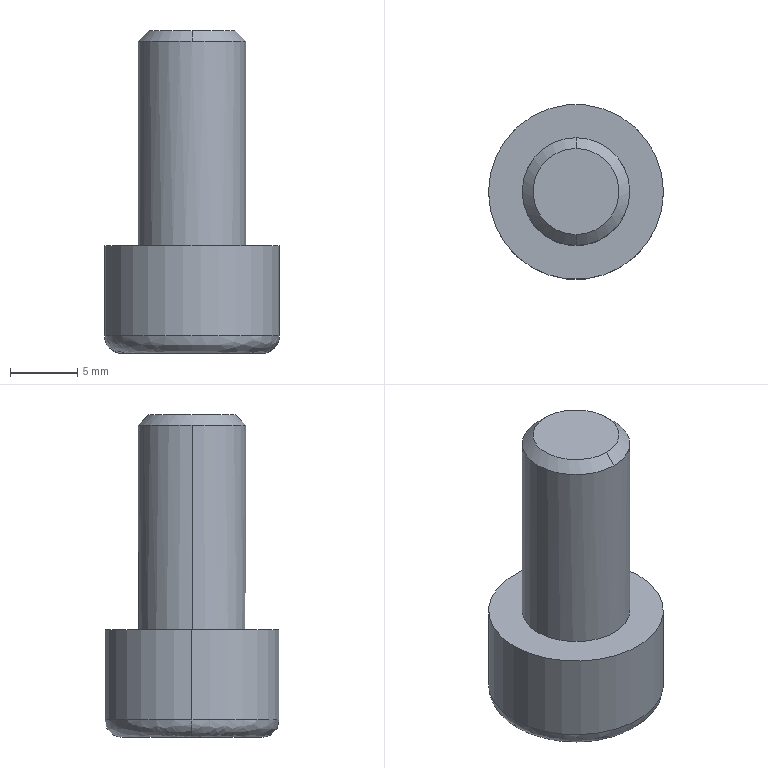Part | STEP file | HJLE-YZS-M8X16_LE0724153021 | 1 solid | 25 faces | box 13 x 13 x 24 mm | volume 1703 mm3 | plane 15 | cylinder 4 | cone 4 | spline 2 | commonest cylinder face diameters 8 x2 13 x2
STEP:
#1=CARTESIAN_POINT('',(-6.5,0.,-6.7));
#2=VERTEX_POINT('',#1);
#3=CARTESIAN_POINT('',(6.5,0.,-6.7));
#4=VERTEX_POINT('',#3);
#5=CARTESIAN_POINT('',(0.,0.,-6.7));
#6=DIRECTION('',(0.,0.,1.));
#7=DIRECTION('',(1.,0.,0.));
#8=AXIS2_PLACEMENT_3D('',#5,#6,#7);
#9=CIRCLE('',#8,6.5);
#10=EDGE_CURVE('',#2,#4,#9,.T.);
#11=ORIENTED_EDGE('',*,*,#10,.F.);
#12=CARTESIAN_POINT('',(-5.2,0.,-8.));
#13=VERTEX_POINT('',#12);
#14=CARTESIAN_POINT('',(-5.2,0.,-6.7));
#15=DIRECTION('',(0.,-1.,0.));
#16=DIRECTION('',(-1.,0.,0.));
#17=AXIS2_PLACEMENT_3D('',#14,#15,#16);
#18=CIRCLE('',#17,1.3);
#19=EDGE_CURVE('',#2,#13,#18,.T.);
#20=ORIENTED_EDGE('',*,*,#19,.T.);
#21=CARTESIAN_POINT('',(5.2,0.,-8.));
#22=VERTEX_POINT('',#21);
#23=CARTESIAN_POINT('',(-5.2,0.,-8.));
#24=CARTESIAN_POINT('',(-5.2,-10.4,-8.));
#25=CARTESIAN_POINT('',(5.2,-10.4,-8.));
#26=CARTESIAN_POINT('',(5.2,0.,-8.));
#27=(BOUNDED_CURVE()B_SPLINE_CURVE(3,(#23,#24,#25,#26),.UNSPECIFIED.,.F.,.F.)B_SPLINE_CURVE_WITH_KNOTS((4,4),(0.,1.),.UNSPECIFIED.)CURVE()GEOMETRIC_REPRESENTATION_ITEM()RATIONAL_B_SPLINE_CURVE((1.,0.3333,0.3333,1.))REPRESENTATION_ITEM(''));
#28=EDGE_CURVE('',#13,#22,#27,.T.);
#29=ORIENTED_EDGE('',*,*,#28,.T.);
#30=CARTESIAN_POINT('',(5.2,0.,-6.7));
#31=DIRECTION('',(0.,1.,0.));
#32=DIRECTION('',(1.,0.,0.));
#33=AXIS2_PLACEMENT_3D('',#30,#31,#32);
#34=CIRCLE('',#33,1.3);
#35=EDGE_CURVE('',#4,#22,#34,.T.);
#36=ORIENTED_EDGE('',*,*,#35,.F.);
#37=EDGE_LOOP('',(#11,#20,#29,#36));
#38=FACE_OUTER_BOUND('',#37,.T.);
#39=CARTESIAN_POINT('',(-6.5,0.,-6.7));
#40=CARTESIAN_POINT('',(-6.5,-13.,-6.7));
#41=CARTESIAN_POINT('',(6.5,-13.,-6.7));
#42=CARTESIAN_POINT('',(6.5,0.,-6.7));
#43=CARTESIAN_POINT('',(-6.5,0.,-7.462));
#44=CARTESIAN_POINT('',(-6.5,-13.,-7.462));
#45=CARTESIAN_POINT('',(6.5,-13.,-7.462));
#46=CARTESIAN_POINT('',(6.5,0.,-7.462));
#47=CARTESIAN_POINT('',(-5.962,0.,-8.));
#48=CARTESIAN_POINT('',(-5.962,-11.923,-8.));
#49=CARTESIAN_POINT('',(5.962,-11.923,-8.));
#50=CARTESIAN_POINT('',(5.962,0.,-8.));
#51=CARTESIAN_POINT('',(-5.2,0.,-8.));
#52=CARTESIAN_POINT('',(-5.2,-10.4,-8.));
#53=CARTESIAN_POINT('',(5.2,-10.4,-8.));
#54=CARTESIAN_POINT('',(5.2,0.,-8.));
#55=(BOUNDED_SURFACE()B_SPLINE_SURFACE(3,3,((#39,#40,#41,#42),(#43,#44,#45,#46),(#47,#48,#49,#50),(#51,#52,#53,#54)),.UNSPECIFIED.,.F.,.F.,.F.)B_SPLINE_SURFACE_WITH_KNOTS((4,4),(4,4),(0.,1.),(0.,1.),.UNSPECIFIED.)GEOMETRIC_REPRESENTATION_ITEM()RATIONAL_B_SPLINE_SURFACE(((1.,0.3333,0.3333,1.),(0.8047,0.2682,0.2682,0.8047),(0.8047,0.2682,0.2682,0.8047),(1.,0.3333,0.3333,1.)))REPRESENTATION_ITEM('')SURFACE());
#56=ADVANCED_FACE('',(#38),#55,.T.);
#57=CARTESIAN_POINT('',(0.,4.,15.2));
#58=VERTEX_POINT('',#57);
#59=CARTESIAN_POINT('',(4.,0.,15.2));
#60=VERTEX_POINT('',#59);
#61=CARTESIAN_POINT('',(0.,0.,15.2));
#62=DIRECTION('',(0.,0.,-1.));
#63=DIRECTION('',(-1.,0.,0.));
#64=AXIS2_PLACEMENT_3D('',#61,#62,#63);
#65=CIRCLE('',#64,4.);
#66=EDGE_CURVE('',#58,#60,#65,.T.);
#67=ORIENTED_EDGE('',*,*,#66,.T.);
#68=CARTESIAN_POINT('',(4.,0.,0.));
#69=VERTEX_POINT('',#68);
#70=CARTESIAN_POINT('',(4.,0.,16.));
#71=DIRECTION('',(0.,0.,-1.));
#72=VECTOR('',#71,1000.);
#73=LINE('',#70,#72);
#74=EDGE_CURVE('',#60,#69,#73,.T.);
#75=ORIENTED_EDGE('',*,*,#74,.T.);
#76=CARTESIAN_POINT('',(-4.,0.,0.));
#77=VERTEX_POINT('',#76);
#78=CARTESIAN_POINT('',(0.,0.,0.));
#79=DIRECTION('',(0.,0.,1.));
#80=DIRECTION('',(-1.,0.,0.));
#81=AXIS2_PLACEMENT_3D('',#78,#79,#80);
#82=CIRCLE('',#81,4.);
#83=EDGE_CURVE('',#69,#77,#82,.T.);
#84=ORIENTED_EDGE('',*,*,#83,.T.);
#85=CARTESIAN_POINT('',(-4.,0.,15.2));
#86=VERTEX_POINT('',#85);
#87=CARTESIAN_POINT('',(-4.,0.,16.));
#88=DIRECTION('',(0.,0.,-1.));
#89=VECTOR('',#88,1000.);
#90=LINE('',#87,#89);
#91=EDGE_CURVE('',#86,#77,#90,.T.);
#92=ORIENTED_EDGE('',*,*,#91,.F.);
#93=CARTESIAN_POINT('',(0.,0.,15.2));
#94=DIRECTION('',(0.,0.,-1.));
#95=DIRECTION('',(-1.,0.,0.));
#96=AXIS2_PLACEMENT_3D('',#93,#94,#95);
#97=CIRCLE('',#96,4.);
#98=EDGE_CURVE('',#86,#58,#97,.T.);
#99=ORIENTED_EDGE('',*,*,#98,.T.);
#100=EDGE_LOOP('',(#67,#75,#84,#92,#99));
#101=FACE_OUTER_BOUND('',#100,.T.);
#102=CARTESIAN_POINT('',(0.,0.,16.));
#103=DIRECTION('',(0.,0.,-1.));
#104=DIRECTION('',(-1.,0.,0.));
#105=AXIS2_PLACEMENT_3D('',#102,#103,#104);
#106=CYLINDRICAL_SURFACE('',#105,4.);
#107=ADVANCED_FACE('',(#101),#106,.T.);
#108=CARTESIAN_POINT('',(0.,3.2,16.));
#109=VERTEX_POINT('',#108);
#110=CARTESIAN_POINT('',(0.,-3.2,16.));
#111=VERTEX_POINT('',#110);
#112=CARTESIAN_POINT('',(0.,0.,16.));
#113=DIRECTION('',(0.,0.,-1.));
#114=DIRECTION('',(0.,1.,0.));
#115=AXIS2_PLACEMENT_3D('',#112,#113,#114);
#116=CIRCLE('',#115,3.2);
#117=EDGE_CURVE('',#109,#111,#116,.T.);
#118=ORIENTED_EDGE('',*,*,#117,.T.);
#119=CARTESIAN_POINT('',(0.,-4.,15.2));
#120=VERTEX_POINT('',#119);
#121=CARTESIAN_POINT('',(0.,-4.,15.2));
#122=DIRECTION('',(0.,-0.7071,-0.7071));
#123=VECTOR('',#122,1000.);
#124=LINE('',#121,#123);
#125=EDGE_CURVE('',#111,#120,#124,.T.);
#126=ORIENTED_EDGE('',*,*,#125,.T.);
#127=CARTESIAN_POINT('',(0.,0.,15.2));
#128=DIRECTION('',(0.,0.,-1.));
#129=DIRECTION('',(-1.,0.,0.));
#130=AXIS2_PLACEMENT_3D('',#127,#128,#129);
#131=CIRCLE('',#130,4.);
#132=EDGE_CURVE('',#60,#120,#131,.T.);
#133=ORIENTED_EDGE('',*,*,#132,.F.);
#134=ORIENTED_EDGE('',*,*,#66,.F.);
#135=CARTESIAN_POINT('',(0.,4.,15.2));
#136=DIRECTION('',(0.,0.7071,-0.7071));
#137=VECTOR('',#136,1000.);
#138=LINE('',#135,#137);
#139=EDGE_CURVE('',#109,#58,#138,.T.);
#140=ORIENTED_EDGE('',*,*,#139,.F.);
#141=EDGE_LOOP('',(#118,#126,#133,#134,#140));
#142=FACE_OUTER_BOUND('',#141,.T.);
#143=CARTESIAN_POINT('',(0.,0.,15.2));
#144=DIRECTION('',(0.,0.,-1.));
#145=DIRECTION('',(0.,1.,0.));
#146=AXIS2_PLACEMENT_3D('',#143,#144,#145);
#147=CONICAL_SURFACE('',#146,4.,0.7854);
#148=ADVANCED_FACE('',(#142),#147,.T.);
#149=CARTESIAN_POINT('',(0.,0.,-6.7));
#150=DIRECTION('',(0.,0.,1.));
#151=DIRECTION('',(1.,0.,0.));
#152=AXIS2_PLACEMENT_3D('',#149,#150,#151);
#153=CIRCLE('',#152,6.5);
#154=EDGE_CURVE('',#4,#2,#153,.T.);
#155=ORIENTED_EDGE('',*,*,#154,.T.);
#156=CARTESIAN_POINT('',(-6.5,0.,0.));
#157=VERTEX_POINT('',#156);
#158=CARTESIAN_POINT('',(-6.5,0.,-8.));
#159=DIRECTION('',(0.,0.,1.));
#160=VECTOR('',#159,1000.);
#161=LINE('',#158,#160);
#162=EDGE_CURVE('',#2,#157,#161,.T.);
#163=ORIENTED_EDGE('',*,*,#162,.T.);
#164=CARTESIAN_POINT('',(6.5,0.,0.));
#165=VERTEX_POINT('',#164);
#166=CARTESIAN_POINT('',(0.,0.,0.));
#167=DIRECTION('',(0.,0.,1.));
#168=DIRECTION('',(1.,0.,0.));
#169=AXIS2_PLACEMENT_3D('',#166,#167,#168);
#170=CIRCLE('',#169,6.5);
#171=EDGE_CURVE('',#165,#157,#170,.T.);
#172=ORIENTED_EDGE('',*,*,#171,.F.);
#173=CARTESIAN_POINT('',(6.5,0.,-8.));
#174=DIRECTION('',(0.,0.,1.));
#175=VECTOR('',#174,1000.);
#176=LINE('',#173,#175);
#177=EDGE_CURVE('',#4,#165,#176,.T.);
#178=ORIENTED_EDGE('',*,*,#177,.F.);
#179=EDGE_LOOP('',(#155,#163,#172,#178));
#180=FACE_OUTER_BOUND('',#179,.T.);
#181=CARTESIAN_POINT('',(0.,0.,-8.));
#182=DIRECTION('',(0.,0.,1.));
#183=DIRECTION('',(1.,0.,0.));
#184=AXIS2_PLACEMENT_3D('',#181,#182,#183);
#185=CYLINDRICAL_SURFACE('',#184,6.5);
#186=ADVANCED_FACE('',(#180),#185,.T.);
#187=CARTESIAN_POINT('',(0.,0.,-2.268));
#188=VERTEX_POINT('',#187);
#189=CARTESIAN_POINT('',(-3.,0.,-4.));
#190=VERTEX_POINT('',#189);
#191=CARTESIAN_POINT('',(-3.,0.,-4.));
#192=DIRECTION('',(-0.866,0.,-0.5));
#193=VECTOR('',#192,1000.);
#194=LINE('',#191,#193);
#195=EDGE_CURVE('',#188,#190,#194,.T.);
#196=ORIENTED_EDGE('',*,*,#195,.F.);
#197=CARTESIAN_POINT('',(3.,0.,-4.));
#198=VERTEX_POINT('',#197);
#199=CARTESIAN_POINT('',(3.,0.,-4.));
#200=DIRECTION('',(0.866,0.,-0.5));
#201=VECTOR('',#200,1000.);
#202=LINE('',#199,#201);
#203=EDGE_CURVE('',#188,#198,#202,.T.);
#204=ORIENTED_EDGE('',*,*,#203,.T.);
#205=CARTESIAN_POINT('',(2.598,-1.5,-4.));
#206=VERTEX_POINT('',#205);
#207=CARTESIAN_POINT('',(0.,0.,-4.));
#208=DIRECTION('',(0.,0.,1.));
#209=DIRECTION('',(-1.,0.,0.));
#210=AXIS2_PLACEMENT_3D('',#207,#208,#209);
#211=CIRCLE('',#210,3.);
#212=EDGE_CURVE('',#206,#198,#211,.T.);
#213=ORIENTED_EDGE('',*,*,#212,.F.);
#214=CARTESIAN_POINT('',(0.,-3.,-4.));
#215=VERTEX_POINT('',#214);
#216=CARTESIAN_POINT('',(0.,0.,-4.));
#217=DIRECTION('',(0.,0.,-1.));
#218=DIRECTION('',(-1.,0.,0.));
#219=AXIS2_PLACEMENT_3D('',#216,#217,#218);
#220=CIRCLE('',#219,3.);
#221=EDGE_CURVE('',#206,#215,#220,.T.);
#222=ORIENTED_EDGE('',*,*,#221,.T.);
#223=CARTESIAN_POINT('',(-2.598,-1.5,-4.));
#224=VERTEX_POINT('',#223);
#225=CARTESIAN_POINT('',(0.,0.,-4.));
#226=DIRECTION('',(0.,0.,1.));
#227=DIRECTION('',(-1.,0.,0.));
#228=AXIS2_PLACEMENT_3D('',#225,#226,#227);
#229=CIRCLE('',#228,3.);
#230=EDGE_CURVE('',#224,#215,#229,.T.);
#231=ORIENTED_EDGE('',*,*,#230,.F.);
#232=CARTESIAN_POINT('',(0.,0.,-4.));
#233=DIRECTION('',(0.,0.,1.));
#234=DIRECTION('',(-1.,0.,0.));
#235=AXIS2_PLACEMENT_3D('',#232,#233,#234);
#236=CIRCLE('',#235,3.);
#237=EDGE_CURVE('',#190,#224,#236,.T.);
#238=ORIENTED_EDGE('',*,*,#237,.F.);
#239=EDGE_LOOP('',(#196,#204,#213,#222,#231,#238));
#240=FACE_OUTER_BOUND('',#239,.T.);
#241=CARTESIAN_POINT('',(0.,0.,-4.));
#242=DIRECTION('',(0.,0.,-1.));
#243=DIRECTION('',(-1.,0.,0.));
#244=AXIS2_PLACEMENT_3D('',#241,#242,#243);
#245=CONICAL_SURFACE('',#244,3.,1.047);
#246=ADVANCED_FACE('',(#240),#245,.F.);
#247=ORIENTED_EDGE('',*,*,#74,.F.);
#248=ORIENTED_EDGE('',*,*,#132,.T.);
#249=CARTESIAN_POINT('',(0.,0.,15.2));
#250=DIRECTION('',(0.,0.,-1.));
#251=DIRECTION('',(-1.,0.,0.));
#252=AXIS2_PLACEMENT_3D('',#249,#250,#251);
#253=CIRCLE('',#252,4.);
#254=EDGE_CURVE('',#120,#86,#253,.T.);
#255=ORIENTED_EDGE('',*,*,#254,.T.);
#256=ORIENTED_EDGE('',*,*,#91,.T.);
#257=CARTESIAN_POINT('',(0.,0.,0.));
#258=DIRECTION('',(0.,0.,1.));
#259=DIRECTION('',(-1.,0.,0.));
#260=AXIS2_PLACEMENT_3D('',#257,#258,#259);
#261=CIRCLE('',#260,4.);
#262=EDGE_CURVE('',#77,#69,#261,.T.);
#263=ORIENTED_EDGE('',*,*,#262,.T.);
#264=EDGE_LOOP('',(#247,#248,#255,#256,#263));
#265=FACE_OUTER_BOUND('',#264,.T.);
#266=CARTESIAN_POINT('',(0.,0.,16.));
#267=DIRECTION('',(0.,0.,-1.));
#268=DIRECTION('',(-1.,0.,0.));
#269=AXIS2_PLACEMENT_3D('',#266,#267,#268);
#270=CYLINDRICAL_SURFACE('',#269,4.);
#271=ADVANCED_FACE('',(#265),#270,.T.);
#272=ORIENTED_EDGE('',*,*,#171,.T.);
#273=CARTESIAN_POINT('',(0.,0.,0.));
#274=DIRECTION('',(0.,0.,1.));
#275=DIRECTION('',(1.,0.,0.));
#276=AXIS2_PLACEMENT_3D('',#273,#274,#275);
#277=CIRCLE('',#276,6.5);
#278=EDGE_CURVE('',#157,#165,#277,.T.);
#279=ORIENTED_EDGE('',*,*,#278,.T.);
#280=EDGE_LOOP('',(#272,#279));
#281=FACE_OUTER_BOUND('',#280,.T.);
#282=ORIENTED_EDGE('',*,*,#262,.F.);
#283=ORIENTED_EDGE('',*,*,#83,.F.);
#284=EDGE_LOOP('',(#282,#283));
#285=FACE_BOUND('',#284,.T.);
#286=CARTESIAN_POINT('',(0.,0.,0.));
#287=DIRECTION('',(0.,0.,1.));
#288=DIRECTION('',(1.,0.,0.));
#289=AXIS2_PLACEMENT_3D('',#286,#287,#288);
#290=PLANE('',#289);
#291=ADVANCED_FACE('',(#281,#285),#290,.T.);
#292=ORIENTED_EDGE('',*,*,#125,.F.);
#293=CARTESIAN_POINT('',(0.,0.,16.));
#294=DIRECTION('',(0.,0.,-1.));
#295=DIRECTION('',(0.,1.,0.));
#296=AXIS2_PLACEMENT_3D('',#293,#294,#295);
#297=CIRCLE('',#296,3.2);
#298=EDGE_CURVE('',#111,#109,#297,.T.);
#299=ORIENTED_EDGE('',*,*,#298,.T.);
#300=ORIENTED_EDGE('',*,*,#139,.T.);
#301=ORIENTED_EDGE('',*,*,#98,.F.);
#302=ORIENTED_EDGE('',*,*,#254,.F.);
#303=EDGE_LOOP('',(#292,#299,#300,#301,#302));
#304=FACE_OUTER_BOUND('',#303,.T.);
#305=CARTESIAN_POINT('',(0.,0.,15.2));
#306=DIRECTION('',(0.,0.,-1.));
#307=DIRECTION('',(0.,1.,0.));
#308=AXIS2_PLACEMENT_3D('',#305,#306,#307);
#309=CONICAL_SURFACE('',#308,4.,0.7854);
#310=ADVANCED_FACE('',(#304),#309,.T.);
#311=ORIENTED_EDGE('',*,*,#162,.F.);
#312=ORIENTED_EDGE('',*,*,#10,.T.);
#313=ORIENTED_EDGE('',*,*,#177,.T.);
#314=ORIENTED_EDGE('',*,*,#278,.F.);
#315=EDGE_LOOP('',(#311,#312,#313,#314));
#316=FACE_OUTER_BOUND('',#315,.T.);
#317=CARTESIAN_POINT('',(0.,0.,-8.));
#318=DIRECTION('',(0.,0.,1.));
#319=DIRECTION('',(1.,0.,0.));
#320=AXIS2_PLACEMENT_3D('',#317,#318,#319);
#321=CYLINDRICAL_SURFACE('',#320,6.5);
#322=ADVANCED_FACE('',(#316),#321,.T.);
#323=ORIENTED_EDGE('',*,*,#117,.F.);
#324=ORIENTED_EDGE('',*,*,#298,.F.);
#325=EDGE_LOOP('',(#323,#324));
#326=FACE_OUTER_BOUND('',#325,.T.);
#327=CARTESIAN_POINT('',(0.,0.,16.));
#328=DIRECTION('',(0.,0.,-1.));
#329=DIRECTION('',(-1.,0.,0.));
#330=AXIS2_PLACEMENT_3D('',#327,#328,#329);
#331=PLANE('',#330);
#332=ADVANCED_FACE('',(#326),#331,.F.);
#333=ORIENTED_EDGE('',*,*,#19,.F.);
#334=ORIENTED_EDGE('',*,*,#154,.F.);
#335=ORIENTED_EDGE('',*,*,#35,.T.);
#336=CARTESIAN_POINT('',(5.2,0.,-8.));
#337=CARTESIAN_POINT('',(5.2,10.4,-8.));
#338=CARTESIAN_POINT('',(-5.2,10.4,-8.));
#339=CARTESIAN_POINT('',(-5.2,0.,-8.));
#340=(BOUNDED_CURVE()B_SPLINE_CURVE(3,(#336,#337,#338,#339),.UNSPECIFIED.,.F.,.F.)B_SPLINE_CURVE_WITH_KNOTS((4,4),(0.,1.),.UNSPECIFIED.)CURVE()GEOMETRIC_REPRESENTATION_ITEM()RATIONAL_B_SPLINE_CURVE((1.,0.3333,0.3333,1.))REPRESENTATION_ITEM(''));
#341=EDGE_CURVE('',#22,#13,#340,.T.);
#342=ORIENTED_EDGE('',*,*,#341,.T.);
#343=EDGE_LOOP('',(#333,#334,#335,#342));
#344=FACE_OUTER_BOUND('',#343,.T.);
#345=CARTESIAN_POINT('',(6.5,0.,-6.7));
#346=CARTESIAN_POINT('',(6.5,13.,-6.7));
#347=CARTESIAN_POINT('',(-6.5,13.,-6.7));
#348=CARTESIAN_POINT('',(-6.5,0.,-6.7));
#349=CARTESIAN_POINT('',(6.5,0.,-7.462));
#350=CARTESIAN_POINT('',(6.5,13.,-7.462));
#351=CARTESIAN_POINT('',(-6.5,13.,-7.462));
#352=CARTESIAN_POINT('',(-6.5,0.,-7.462));
#353=CARTESIAN_POINT('',(5.962,0.,-8.));
#354=CARTESIAN_POINT('',(5.962,11.923,-8.));
#355=CARTESIAN_POINT('',(-5.962,11.923,-8.));
#356=CARTESIAN_POINT('',(-5.962,0.,-8.));
#357=CARTESIAN_POINT('',(5.2,0.,-8.));
#358=CARTESIAN_POINT('',(5.2,10.4,-8.));
#359=CARTESIAN_POINT('',(-5.2,10.4,-8.));
#360=CARTESIAN_POINT('',(-5.2,0.,-8.));
#361=(BOUNDED_SURFACE()B_SPLINE_SURFACE(3,3,((#345,#346,#347,#348),(#349,#350,#351,#352),(#353,#354,#355,#356),(#357,#358,#359,#360)),.UNSPECIFIED.,.F.,.F.,.T.)B_SPLINE_SURFACE_WITH_KNOTS((4,4),(4,4),(0.,1.),(0.,1.),.UNSPECIFIED.)GEOMETRIC_REPRESENTATION_ITEM()RATIONAL_B_SPLINE_SURFACE(((1.,0.3333,0.3333,1.),(0.8047,0.2682,0.2682,0.8047),(0.8047,0.2682,0.2682,0.8047),(1.,0.3333,0.3333,1.)))REPRESENTATION_ITEM('')SURFACE());
#362=ADVANCED_FACE('',(#344),#361,.T.);
#363=CARTESIAN_POINT('',(-1.732,3.,-8.));
#364=VERTEX_POINT('',#363);
#365=CARTESIAN_POINT('',(1.732,3.,-8.));
#366=VERTEX_POINT('',#365);
#367=CARTESIAN_POINT('',(0.,3.,-8.));
#368=DIRECTION('',(1.,0.,0.));
#369=VECTOR('',#368,1000.);
#370=LINE('',#367,#369);
#371=EDGE_CURVE('',#364,#366,#370,.T.);
#372=ORIENTED_EDGE('',*,*,#371,.F.);
#373=CARTESIAN_POINT('',(-3.464,0.,-8.));
#374=VERTEX_POINT('',#373);
#375=CARTESIAN_POINT('',(-3.464,0.,-8.));
#376=DIRECTION('',(0.5,0.866,0.));
#377=VECTOR('',#376,1000.);
#378=LINE('',#375,#377);
#379=EDGE_CURVE('',#374,#364,#378,.T.);
#380=ORIENTED_EDGE('',*,*,#379,.F.);
#381=CARTESIAN_POINT('',(-1.732,-3.,-8.));
#382=VERTEX_POINT('',#381);
#383=CARTESIAN_POINT('',(-1.732,-3.,-8.));
#384=DIRECTION('',(-0.5,0.866,0.));
#385=VECTOR('',#384,1000.);
#386=LINE('',#383,#385);
#387=EDGE_CURVE('',#382,#374,#386,.T.);
#388=ORIENTED_EDGE('',*,*,#387,.F.);
#389=CARTESIAN_POINT('',(1.732,-3.,-8.));
#390=VERTEX_POINT('',#389);
#391=CARTESIAN_POINT('',(0.,-3.,-8.));
#392=DIRECTION('',(-1.,0.,0.));
#393=VECTOR('',#392,1000.);
#394=LINE('',#391,#393);
#395=EDGE_CURVE('',#390,#382,#394,.T.);
#396=ORIENTED_EDGE('',*,*,#395,.F.);
#397=CARTESIAN_POINT('',(3.464,0.,-8.));
#398=VERTEX_POINT('',#397);
#399=CARTESIAN_POINT('',(3.464,0.,-8.));
#400=DIRECTION('',(-0.5,-0.866,0.));
#401=VECTOR('',#400,1000.);
#402=LINE('',#399,#401);
#403=EDGE_CURVE('',#398,#390,#402,.T.);
#404=ORIENTED_EDGE('',*,*,#403,.F.);
#405=CARTESIAN_POINT('',(1.732,3.,-8.));
#406=DIRECTION('',(0.5,-0.866,0.));
#407=VECTOR('',#406,1000.);
#408=LINE('',#405,#407);
#409=EDGE_CURVE('',#366,#398,#408,.T.);
#410=ORIENTED_EDGE('',*,*,#409,.F.);
#411=EDGE_LOOP('',(#372,#380,#388,#396,#404,#410));
#412=FACE_BOUND('',#411,.T.);
#413=ORIENTED_EDGE('',*,*,#341,.F.);
#414=ORIENTED_EDGE('',*,*,#28,.F.);
#415=EDGE_LOOP('',(#413,#414));
#416=FACE_OUTER_BOUND('',#415,.T.);
#417=CARTESIAN_POINT('',(0.,0.,-8.));
#418=DIRECTION('',(0.,0.,1.));
#419=DIRECTION('',(1.,0.,0.));
#420=AXIS2_PLACEMENT_3D('',#417,#418,#419);
#421=PLANE('',#420);
#422=ADVANCED_FACE('',(#412,#416),#421,.F.);
#423=CARTESIAN_POINT('',(2.598,1.5,-4.));
#424=VERTEX_POINT('',#423);
#425=CARTESIAN_POINT('',(1.732,3.,-4.));
#426=VERTEX_POINT('',#425);
#427=CARTESIAN_POINT('',(2.598,1.5,-4.));
#428=DIRECTION('',(-0.5,0.866,0.));
#429=VECTOR('',#428,1000.);
#430=LINE('',#427,#429);
#431=EDGE_CURVE('',#424,#426,#430,.T.);
#432=ORIENTED_EDGE('',*,*,#431,.T.);
#433=CARTESIAN_POINT('',(1.732,3.,-4.));
#434=DIRECTION('',(0.,0.,-1.));
#435=VECTOR('',#434,1000.);
#436=LINE('',#433,#435);
#437=EDGE_CURVE('',#426,#366,#436,.T.);
#438=ORIENTED_EDGE('',*,*,#437,.T.);
#439=ORIENTED_EDGE('',*,*,#409,.T.);
#440=CARTESIAN_POINT('',(3.464,0.,-4.));
#441=VERTEX_POINT('',#440);
#442=CARTESIAN_POINT('',(3.464,0.,-4.));
#443=DIRECTION('',(0.,0.,1.));
#444=VECTOR('',#443,1000.);
#445=LINE('',#442,#444);
#446=EDGE_CURVE('',#398,#441,#445,.T.);
#447=ORIENTED_EDGE('',*,*,#446,.T.);
#448=CARTESIAN_POINT('',(3.464,0.,-4.));
#449=DIRECTION('',(-0.5,0.866,0.));
#450=VECTOR('',#449,1000.);
#451=LINE('',#448,#450);
#452=EDGE_CURVE('',#441,#424,#451,.T.);
#453=ORIENTED_EDGE('',*,*,#452,.T.);
#454=EDGE_LOOP('',(#432,#438,#439,#447,#453));
#455=FACE_OUTER_BOUND('',#454,.T.);
#456=CARTESIAN_POINT('',(3.464,0.,-4.));
#457=DIRECTION('',(-0.866,-0.5,0.));
#458=DIRECTION('',(0.5,-0.866,0.));
#459=AXIS2_PLACEMENT_3D('',#456,#457,#458);
#460=PLANE('',#459);
#461=ADVANCED_FACE('',(#455),#460,.T.);
#462=CARTESIAN_POINT('',(0.,3.,-4.));
#463=VERTEX_POINT('',#462);
#464=CARTESIAN_POINT('',(-1.732,3.,-4.));
#465=VERTEX_POINT('',#464);
#466=CARTESIAN_POINT('',(0.,3.,-4.));
#467=DIRECTION('',(-1.,0.,0.));
#468=VECTOR('',#467,1000.);
#469=LINE('',#466,#468);
#470=EDGE_CURVE('',#463,#465,#469,.T.);
#471=ORIENTED_EDGE('',*,*,#470,.T.);
#472=CARTESIAN_POINT('',(-1.732,3.,-4.));
#473=DIRECTION('',(0.,0.,-1.));
#474=VECTOR('',#473,1000.);
#475=LINE('',#472,#474);
#476=EDGE_CURVE('',#465,#364,#475,.T.);
#477=ORIENTED_EDGE('',*,*,#476,.T.);
#478=ORIENTED_EDGE('',*,*,#371,.T.);
#479=ORIENTED_EDGE('',*,*,#437,.F.);
#480=CARTESIAN_POINT('',(0.,3.,-4.));
#481=DIRECTION('',(-1.,0.,0.));
#482=VECTOR('',#481,1000.);
#483=LINE('',#480,#482);
#484=EDGE_CURVE('',#426,#463,#483,.T.);
#485=ORIENTED_EDGE('',*,*,#484,.T.);
#486=EDGE_LOOP('',(#471,#477,#478,#479,#485));
#487=FACE_OUTER_BOUND('',#486,.T.);
#488=CARTESIAN_POINT('',(1.732,3.,-4.));
#489=DIRECTION('',(0.,-1.,0.));
#490=DIRECTION('',(1.,0.,0.));
#491=AXIS2_PLACEMENT_3D('',#488,#489,#490);
#492=PLANE('',#491);
#493=ADVANCED_FACE('',(#487),#492,.T.);
#494=CARTESIAN_POINT('',(-2.598,1.5,-4.));
#495=VERTEX_POINT('',#494);
#496=CARTESIAN_POINT('',(-3.464,0.,-4.));
#497=VERTEX_POINT('',#496);
#498=CARTESIAN_POINT('',(-1.732,3.,-4.));
#499=DIRECTION('',(-0.5,-0.866,0.));
#500=VECTOR('',#499,1000.);
#501=LINE('',#498,#500);
#502=EDGE_CURVE('',#495,#497,#501,.T.);
#503=ORIENTED_EDGE('',*,*,#502,.T.);
#504=CARTESIAN_POINT('',(-3.464,0.,-4.));
#505=DIRECTION('',(0.,0.,-1.));
#506=VECTOR('',#505,1000.);
#507=LINE('',#504,#506);
#508=EDGE_CURVE('',#497,#374,#507,.T.);
#509=ORIENTED_EDGE('',*,*,#508,.T.);
#510=ORIENTED_EDGE('',*,*,#379,.T.);
#511=ORIENTED_EDGE('',*,*,#476,.F.);
#512=CARTESIAN_POINT('',(-1.732,3.,-4.));
#513=DIRECTION('',(-0.5,-0.866,0.));
#514=VECTOR('',#513,1000.);
#515=LINE('',#512,#514);
#516=EDGE_CURVE('',#465,#495,#515,.T.);
#517=ORIENTED_EDGE('',*,*,#516,.T.);
#518=EDGE_LOOP('',(#503,#509,#510,#511,#517));
#519=FACE_OUTER_BOUND('',#518,.T.);
#520=CARTESIAN_POINT('',(-1.732,3.,-4.));
#521=DIRECTION('',(0.866,-0.5,0.));
#522=DIRECTION('',(0.5,0.866,0.));
#523=AXIS2_PLACEMENT_3D('',#520,#521,#522);
#524=PLANE('',#523);
#525=ADVANCED_FACE('',(#519),#524,.T.);
#526=CARTESIAN_POINT('',(-1.732,-3.,-4.));
#527=VERTEX_POINT('',#526);
#528=CARTESIAN_POINT('',(-2.598,-1.5,-4.));
#529=DIRECTION('',(0.5,-0.866,0.));
#530=VECTOR('',#529,1000.);
#531=LINE('',#528,#530);
#532=EDGE_CURVE('',#224,#527,#531,.T.);
#533=ORIENTED_EDGE('',*,*,#532,.T.);
#534=CARTESIAN_POINT('',(-1.732,-3.,-4.));
#535=DIRECTION('',(0.,0.,-1.));
#536=VECTOR('',#535,1000.);
#537=LINE('',#534,#536);
#538=EDGE_CURVE('',#527,#382,#537,.T.);
#539=ORIENTED_EDGE('',*,*,#538,.T.);
#540=ORIENTED_EDGE('',*,*,#387,.T.);
#541=ORIENTED_EDGE('',*,*,#508,.F.);
#542=CARTESIAN_POINT('',(-3.464,0.,-4.));
#543=DIRECTION('',(0.5,-0.866,0.));
#544=VECTOR('',#543,1000.);
#545=LINE('',#542,#544);
#546=EDGE_CURVE('',#497,#224,#545,.T.);
#547=ORIENTED_EDGE('',*,*,#546,.T.);
#548=EDGE_LOOP('',(#533,#539,#540,#541,#547));
#549=FACE_OUTER_BOUND('',#548,.T.);
#550=CARTESIAN_POINT('',(-3.464,0.,-4.));
#551=DIRECTION('',(0.866,0.5,0.));
#552=DIRECTION('',(-0.5,0.866,0.));
#553=AXIS2_PLACEMENT_3D('',#550,#551,#552);
#554=PLANE('',#553);
#555=ADVANCED_FACE('',(#549),#554,.T.);
#556=CARTESIAN_POINT('',(1.732,-3.,-4.));
#557=VERTEX_POINT('',#556);
#558=CARTESIAN_POINT('',(-1.732,-3.,-4.));
#559=DIRECTION('',(1.,0.,0.));
#560=VECTOR('',#559,1000.);
#561=LINE('',#558,#560);
#562=EDGE_CURVE('',#215,#557,#561,.T.);
#563=ORIENTED_EDGE('',*,*,#562,.T.);
#564=CARTESIAN_POINT('',(1.732,-3.,-4.));
#565=DIRECTION('',(0.,0.,-1.));
#566=VECTOR('',#565,1000.);
#567=LINE('',#564,#566);
#568=EDGE_CURVE('',#557,#390,#567,.T.);
#569=ORIENTED_EDGE('',*,*,#568,.T.);
#570=ORIENTED_EDGE('',*,*,#395,.T.);
#571=ORIENTED_EDGE('',*,*,#538,.F.);
#572=CARTESIAN_POINT('',(0.,-3.,-4.));
#573=DIRECTION('',(1.,0.,0.));
#574=VECTOR('',#573,1000.);
#575=LINE('',#572,#574);
#576=EDGE_CURVE('',#527,#215,#575,.T.);
#577=ORIENTED_EDGE('',*,*,#576,.T.);
#578=EDGE_LOOP('',(#563,#569,#570,#571,#577));
#579=FACE_OUTER_BOUND('',#578,.T.);
#580=CARTESIAN_POINT('',(-1.732,-3.,-4.));
#581=DIRECTION('',(0.,1.,0.));
#582=DIRECTION('',(0.,0.,1.));
#583=AXIS2_PLACEMENT_3D('',#580,#581,#582);
#584=PLANE('',#583);
#585=ADVANCED_FACE('',(#579),#584,.T.);
#586=CARTESIAN_POINT('',(1.732,-3.,-4.));
#587=DIRECTION('',(0.5,0.866,0.));
#588=VECTOR('',#587,1000.);
#589=LINE('',#586,#588);
#590=EDGE_CURVE('',#206,#441,#589,.T.);
#591=ORIENTED_EDGE('',*,*,#590,.T.);
#592=ORIENTED_EDGE('',*,*,#446,.F.);
#593=ORIENTED_EDGE('',*,*,#403,.T.);
#594=ORIENTED_EDGE('',*,*,#568,.F.);
#595=CARTESIAN_POINT('',(1.732,-3.,-4.));
#596=DIRECTION('',(0.5,0.866,0.));
#597=VECTOR('',#596,1000.);
#598=LINE('',#595,#597);
#599=EDGE_CURVE('',#557,#206,#598,.T.);
#600=ORIENTED_EDGE('',*,*,#599,.T.);
#601=EDGE_LOOP('',(#591,#592,#593,#594,#600));
#602=FACE_OUTER_BOUND('',#601,.T.);
#603=CARTESIAN_POINT('',(1.732,-3.,-4.));
#604=DIRECTION('',(-0.866,0.5,0.));
#605=DIRECTION('',(-0.5,-0.866,0.));
#606=AXIS2_PLACEMENT_3D('',#603,#604,#605);
#607=PLANE('',#606);
#608=ADVANCED_FACE('',(#602),#607,.T.);
#609=ORIENTED_EDGE('',*,*,#212,.T.);
#610=CARTESIAN_POINT('',(0.,0.,-4.));
#611=DIRECTION('',(0.,0.,1.));
#612=DIRECTION('',(-1.,0.,0.));
#613=AXIS2_PLACEMENT_3D('',#610,#611,#612);
#614=CIRCLE('',#613,3.);
#615=EDGE_CURVE('',#198,#424,#614,.T.);
#616=ORIENTED_EDGE('',*,*,#615,.T.);
#617=ORIENTED_EDGE('',*,*,#452,.F.);
#618=ORIENTED_EDGE('',*,*,#590,.F.);
#619=EDGE_LOOP('',(#609,#616,#617,#618));
#620=FACE_OUTER_BOUND('',#619,.T.);
#621=CARTESIAN_POINT('',(0.,0.,-4.));
#622=DIRECTION('',(0.,0.,1.));
#623=DIRECTION('',(1.,0.,0.));
#624=AXIS2_PLACEMENT_3D('',#621,#622,#623);
#625=PLANE('',#624);
#626=ADVANCED_FACE('',(#620),#625,.F.);
#627=ORIENTED_EDGE('',*,*,#502,.F.);
#628=CARTESIAN_POINT('',(0.,0.,-4.));
#629=DIRECTION('',(0.,0.,1.));
#630=DIRECTION('',(-1.,0.,0.));
#631=AXIS2_PLACEMENT_3D('',#628,#629,#630);
#632=CIRCLE('',#631,3.);
#633=EDGE_CURVE('',#495,#190,#632,.T.);
#634=ORIENTED_EDGE('',*,*,#633,.T.);
#635=ORIENTED_EDGE('',*,*,#237,.T.);
#636=ORIENTED_EDGE('',*,*,#546,.F.);
#637=EDGE_LOOP('',(#627,#634,#635,#636));
#638=FACE_OUTER_BOUND('',#637,.T.);
#639=CARTESIAN_POINT('',(0.,0.,-4.));
#640=DIRECTION('',(0.,0.,1.));
#641=DIRECTION('',(1.,0.,0.));
#642=AXIS2_PLACEMENT_3D('',#639,#640,#641);
#643=PLANE('',#642);
#644=ADVANCED_FACE('',(#638),#643,.F.);
#645=ORIENTED_EDGE('',*,*,#221,.F.);
#646=ORIENTED_EDGE('',*,*,#599,.F.);
#647=ORIENTED_EDGE('',*,*,#562,.F.);
#648=EDGE_LOOP('',(#645,#646,#647));
#649=FACE_OUTER_BOUND('',#648,.T.);
#650=CARTESIAN_POINT('',(0.,0.,-4.));
#651=DIRECTION('',(0.,0.,1.));
#652=DIRECTION('',(1.,0.,0.));
#653=AXIS2_PLACEMENT_3D('',#650,#651,#652);
#654=PLANE('',#653);
#655=ADVANCED_FACE('',(#649),#654,.F.);
#656=ORIENTED_EDGE('',*,*,#203,.F.);
#657=ORIENTED_EDGE('',*,*,#195,.T.);
#658=ORIENTED_EDGE('',*,*,#633,.F.);
#659=CARTESIAN_POINT('',(0.,0.,-4.));
#660=DIRECTION('',(0.,0.,1.));
#661=DIRECTION('',(-1.,0.,0.));
#662=AXIS2_PLACEMENT_3D('',#659,#660,#661);
#663=CIRCLE('',#662,3.);
#664=EDGE_CURVE('',#463,#495,#663,.T.);
#665=ORIENTED_EDGE('',*,*,#664,.F.);
#666=CARTESIAN_POINT('',(0.,0.,-4.));
#667=DIRECTION('',(0.,0.,1.));
#668=DIRECTION('',(-1.,0.,0.));
#669=AXIS2_PLACEMENT_3D('',#666,#667,#668);
#670=CIRCLE('',#669,3.);
#671=EDGE_CURVE('',#424,#463,#670,.T.);
#672=ORIENTED_EDGE('',*,*,#671,.F.);
#673=ORIENTED_EDGE('',*,*,#615,.F.);
#674=EDGE_LOOP('',(#656,#657,#658,#665,#672,#673));
#675=FACE_OUTER_BOUND('',#674,.T.);
#676=CARTESIAN_POINT('',(0.,0.,-4.));
#677=DIRECTION('',(0.,0.,-1.));
#678=DIRECTION('',(-1.,0.,0.));
#679=AXIS2_PLACEMENT_3D('',#676,#677,#678);
#680=CONICAL_SURFACE('',#679,3.,1.047);
#681=ADVANCED_FACE('',(#675),#680,.F.);
#682=ORIENTED_EDGE('',*,*,#230,.T.);
#683=ORIENTED_EDGE('',*,*,#576,.F.);
#684=ORIENTED_EDGE('',*,*,#532,.F.);
#685=EDGE_LOOP('',(#682,#683,#684));
#686=FACE_OUTER_BOUND('',#685,.T.);
#687=CARTESIAN_POINT('',(0.,0.,-4.));
#688=DIRECTION('',(0.,0.,1.));
#689=DIRECTION('',(1.,0.,0.));
#690=AXIS2_PLACEMENT_3D('',#687,#688,#689);
#691=PLANE('',#690);
#692=ADVANCED_FACE('',(#686),#691,.F.);
#693=ORIENTED_EDGE('',*,*,#664,.T.);
#694=ORIENTED_EDGE('',*,*,#516,.F.);
#695=ORIENTED_EDGE('',*,*,#470,.F.);
#696=EDGE_LOOP('',(#693,#694,#695));
#697=FACE_OUTER_BOUND('',#696,.T.);
#698=CARTESIAN_POINT('',(0.,0.,-4.));
#699=DIRECTION('',(0.,0.,1.));
#700=DIRECTION('',(1.,0.,0.));
#701=AXIS2_PLACEMENT_3D('',#698,#699,#700);
#702=PLANE('',#701);
#703=ADVANCED_FACE('',(#697),#702,.F.);
#704=ORIENTED_EDGE('',*,*,#671,.T.);
#705=ORIENTED_EDGE('',*,*,#484,.F.);
#706=ORIENTED_EDGE('',*,*,#431,.F.);
#707=EDGE_LOOP('',(#704,#705,#706));
#708=FACE_OUTER_BOUND('',#707,.T.);
#709=CARTESIAN_POINT('',(0.,0.,-4.));
#710=DIRECTION('',(0.,0.,1.));
#711=DIRECTION('',(1.,0.,0.));
#712=AXIS2_PLACEMENT_3D('',#709,#710,#711);
#713=PLANE('',#712);
#714=ADVANCED_FACE('',(#708),#713,.F.);
#715=CLOSED_SHELL('',(#56,#107,#148,#186,#246,#271,#291,#310,#322,#332,#362,#422,#461,#493,#525,#555,#585,#608,#626,#644,#655,#681,#692,#703,#714));
#716=MANIFOLD_SOLID_BREP('',#715);
#717=CARTESIAN_POINT('',(0.,0.,0.));
#718=DIRECTION('',(0.,0.,1.));
#719=DIRECTION('',(1.,0.,0.));
#720=AXIS2_PLACEMENT_3D('',#717,#718,#719);
#721=(LENGTH_UNIT()NAMED_UNIT(*)SI_UNIT(.MILLI.,.METRE.));
#722=UNCERTAINTY_MEASURE_WITH_UNIT(LENGTH_MEASURE(0.00001),#721,'','');
#723=(NAMED_UNIT(*)PLANE_ANGLE_UNIT()SI_UNIT($,.RADIAN.));
#724=(NAMED_UNIT(*)SI_UNIT($,.STERADIAN.)SOLID_ANGLE_UNIT());
#725=(GEOMETRIC_REPRESENTATION_CONTEXT(3)GLOBAL_UNCERTAINTY_ASSIGNED_CONTEXT((#722))GLOBAL_UNIT_ASSIGNED_CONTEXT((#721,#723,#724))REPRESENTATION_CONTEXT('',''));
#726=ADVANCED_BREP_SHAPE_REPRESENTATION('',(#716,#720),#725);